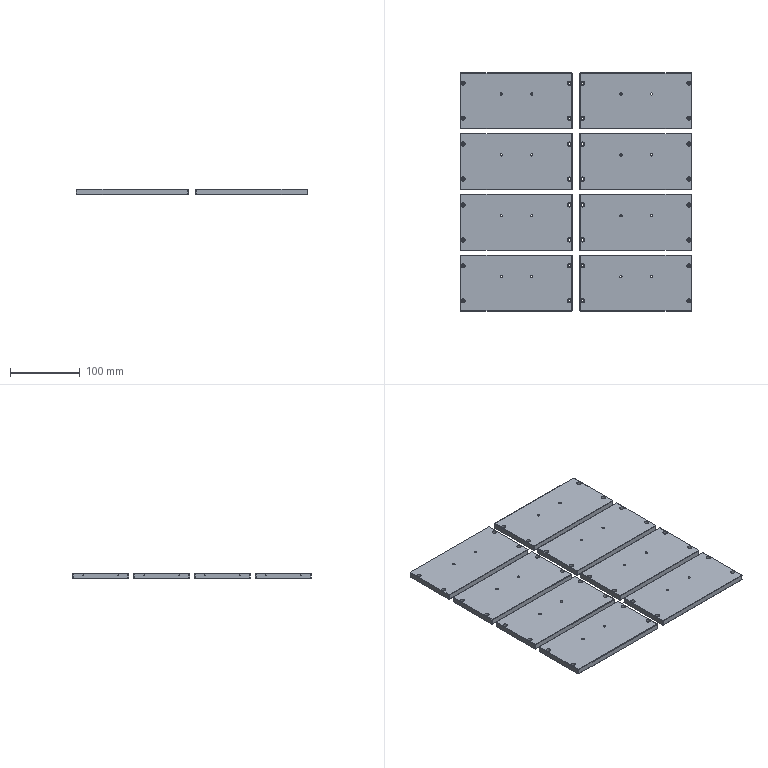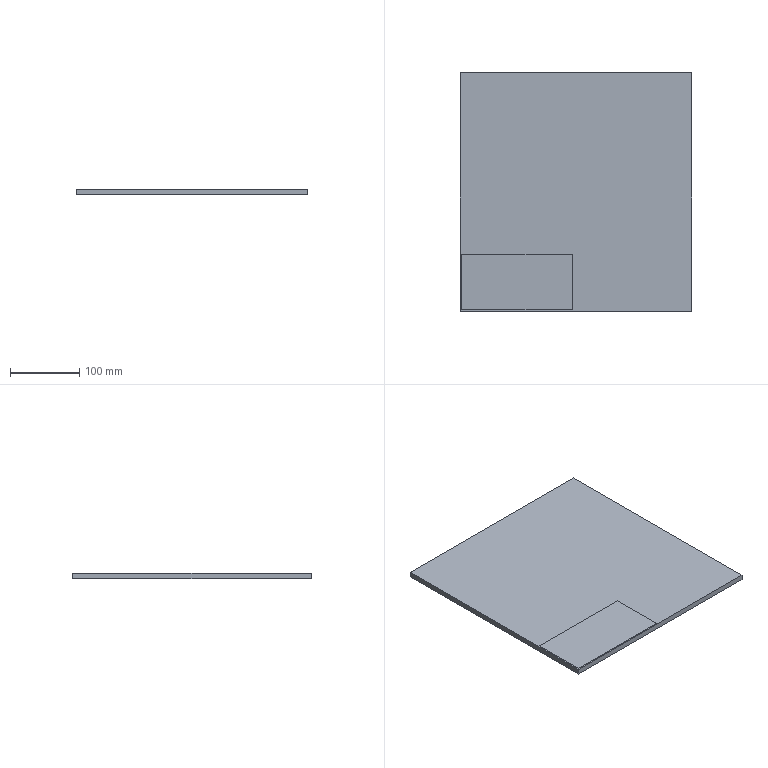CAM job | NX | 3-axis milling, drilling | part box 331 x 341 x 8 mm | stock box 335 x 345 x 8 mm
Tools:
number,name,description,diameter,corner_radius,flute_length,length,flutes
2,D4A45,Milling Tool-5 Parameters,4.0,0.0,2.0,2.0,2
4,D4,Milling Tool-5 Parameters,4.0,0.0,50.0,75.0,2
6,D6,Milling Tool-5 Parameters,6.0,0.0,50.0,75.0,2
15,3.5ZT,Drilling Tool,3.5,0.0,35.0,50.0,2
13,3.3ZT,Drilling Tool,3.3,0.0,35.0,50.0,2
Operations:
program,operation,operation_type,tool,method,geometry_group,spindle_rpm,surface_speed,feed_per_tooth,feed_cut,feed_plunge,cut_length_mm,path_length_mm,cut_time_min,machine_time_min
1吸,ZLEVEL_PROFILE_1_COPY_1_COPY,ZLevelMilling,D4A45,METHOD,A,9500.0,179.0,0.0526,1000.0,100.0,4584.268,14949.959,4.584,5.621
1吸,HOLE_MILLING,CylinderMilling,D4,METHOD,A,9500.0,179.0,0.1158,2200.0,100.0,2487.865,6023.365,1.131,1.484
1吸,ZLEVEL_PROFILE_COPY_COPY_1_COPY,ZLevelMilling,D6,METHOD,A,9500.0,179.0,0.1158,2200.0,1000.0,64248.396,66105.127,29.369,29.555
1吸,ZLEVEL_PROFILE_COPY_COPY_COPY_COPY,ZLevelMilling,D6,MILL_FINISH,A,9500.0,119.0,0.0632,1200.0,1000.0,4021.524,6513.337,3.355,3.604
2,DRILLING_COPY,Operation,D4A45,METHOD,B,5000.0,62.0,0.025,250.0,0.0,21.6,374.988,0.0864,0.1217
2,DRILLING_COPY_COPY_COPY_COPY_COPY,Operation,3.5ZT,METHOD,B,1910.0,21.0,0.0471,180.0,0.0,38.206,617.523,0.2123,0.2702
2,DRILLING_COPY_COPY_COPY_COPY_COPY_COPY,Operation,3.3ZT,METHOD,B,1910.0,21.0,0.0471,180.0,0.0,26.983,160.669,0.1499,0.1633
2,ZLEVEL_PROFILE_1_COPY_1_COPY_COPY,ZLevelMilling,D4A45,METHOD,B,9500.0,179.0,0.0526,1000.0,100.0,534.374,1623.745,0.5344,0.6433